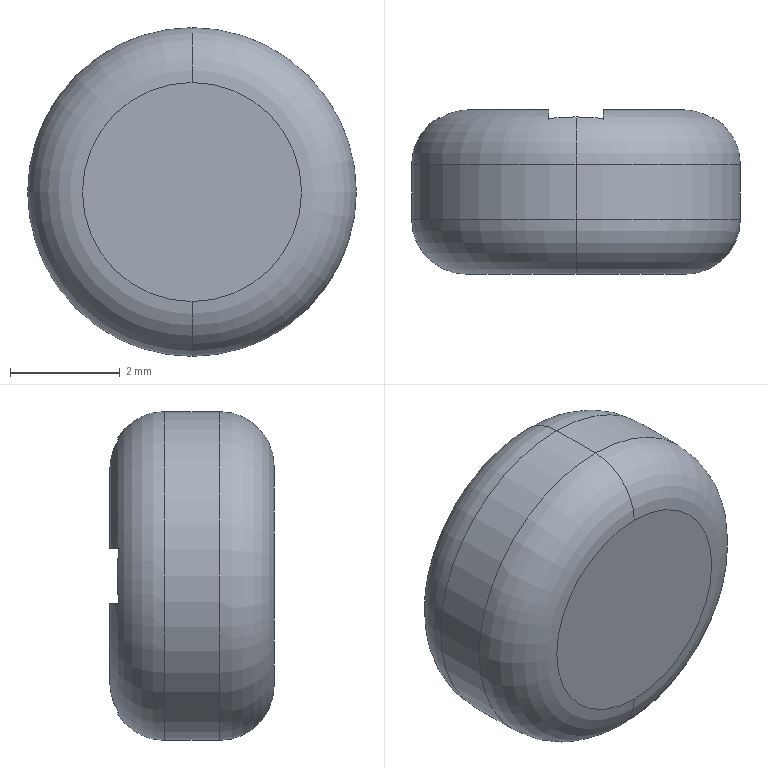Part | SolidWorks | features BaseBody 1 | 1 solid | 24 faces | box 6 x 3 x 6 mm | volume 63.932 mm3 | plane 18 | torus 4 | cylinder 2 | commonest cylinder face diameters 6 x2
STEP:
#1=CARTESIAN_POINT('',(0.,0.,-2.));
#2=VERTEX_POINT('',#1);
#3=CARTESIAN_POINT('',(0.,0.,2.));
#4=VERTEX_POINT('',#3);
#5=CARTESIAN_POINT('',(0.,0.,0.));
#6=DIRECTION('',(0.,-1.,0.));
#7=DIRECTION('',(0.,0.,1.));
#8=AXIS2_PLACEMENT_3D('',#5,#6,#7);
#9=CIRCLE('',#8,2.);
#10=EDGE_CURVE('',#2,#4,#9,.T.);
#11=ORIENTED_EDGE('',*,*,#10,.F.);
#12=CARTESIAN_POINT('',(0.,1.,-3.));
#13=VERTEX_POINT('',#12);
#14=CARTESIAN_POINT('',(0.,1.,-2.));
#15=DIRECTION('',(1.,0.,0.));
#16=DIRECTION('',(0.,0.,-1.));
#17=AXIS2_PLACEMENT_3D('',#14,#15,#16);
#18=CIRCLE('',#17,1.);
#19=EDGE_CURVE('',#2,#13,#18,.T.);
#20=ORIENTED_EDGE('',*,*,#19,.T.);
#21=CARTESIAN_POINT('',(0.,1.,3.));
#22=VERTEX_POINT('',#21);
#23=CARTESIAN_POINT('',(0.,1.,0.));
#24=DIRECTION('',(0.,1.,0.));
#25=DIRECTION('',(0.,0.,1.));
#26=AXIS2_PLACEMENT_3D('',#23,#24,#25);
#27=CIRCLE('',#26,3.);
#28=EDGE_CURVE('',#22,#13,#27,.T.);
#29=ORIENTED_EDGE('',*,*,#28,.F.);
#30=CARTESIAN_POINT('',(0.,1.,2.));
#31=DIRECTION('',(-1.,0.,0.));
#32=DIRECTION('',(0.,0.,1.));
#33=AXIS2_PLACEMENT_3D('',#30,#31,#32);
#34=CIRCLE('',#33,1.);
#35=EDGE_CURVE('',#4,#22,#34,.T.);
#36=ORIENTED_EDGE('',*,*,#35,.F.);
#37=EDGE_LOOP('',(#11,#20,#29,#36));
#38=FACE_OUTER_BOUND('',#37,.T.);
#39=CARTESIAN_POINT('',(0.,1.,0.));
#40=DIRECTION('',(0.,1.,0.));
#41=DIRECTION('',(0.,0.,1.));
#42=AXIS2_PLACEMENT_3D('',#39,#40,#41);
#43=TOROIDAL_SURFACE('',#42,2.,1.);
#44=ADVANCED_FACE('',(#38),#43,.T.);
#45=CARTESIAN_POINT('',(0.,2.,-3.));
#46=VERTEX_POINT('',#45);
#47=CARTESIAN_POINT('',(0.,2.,3.));
#48=VERTEX_POINT('',#47);
#49=CARTESIAN_POINT('',(0.,2.,0.));
#50=DIRECTION('',(0.,-1.,0.));
#51=DIRECTION('',(0.,0.,1.));
#52=AXIS2_PLACEMENT_3D('',#49,#50,#51);
#53=CIRCLE('',#52,3.);
#54=EDGE_CURVE('',#46,#48,#53,.T.);
#55=ORIENTED_EDGE('',*,*,#54,.T.);
#56=CARTESIAN_POINT('',(0.,3.,3.));
#57=DIRECTION('',(0.,-1.,0.));
#58=VECTOR('',#57,1000.);
#59=LINE('',#56,#58);
#60=EDGE_CURVE('',#48,#22,#59,.T.);
#61=ORIENTED_EDGE('',*,*,#60,.T.);
#62=ORIENTED_EDGE('',*,*,#28,.T.);
#63=CARTESIAN_POINT('',(0.,3.,-3.));
#64=DIRECTION('',(0.,-1.,0.));
#65=VECTOR('',#64,1000.);
#66=LINE('',#63,#65);
#67=EDGE_CURVE('',#46,#13,#66,.T.);
#68=ORIENTED_EDGE('',*,*,#67,.F.);
#69=EDGE_LOOP('',(#55,#61,#62,#68));
#70=FACE_OUTER_BOUND('',#69,.T.);
#71=CARTESIAN_POINT('',(0.,3.,0.));
#72=DIRECTION('',(0.,-1.,0.));
#73=DIRECTION('',(0.,0.,-1.));
#74=AXIS2_PLACEMENT_3D('',#71,#72,#73);
#75=CYLINDRICAL_SURFACE('',#74,3.);
#76=ADVANCED_FACE('',(#70),#75,.T.);
#77=ORIENTED_EDGE('',*,*,#54,.F.);
#78=CARTESIAN_POINT('',(0.,2.866,-2.5));
#79=VERTEX_POINT('',#78);
#80=CARTESIAN_POINT('',(0.,2.,-2.));
#81=DIRECTION('',(1.,0.,0.));
#82=DIRECTION('',(0.,0.,-1.));
#83=AXIS2_PLACEMENT_3D('',#80,#81,#82);
#84=CIRCLE('',#83,1.);
#85=EDGE_CURVE('',#46,#79,#84,.T.);
#86=ORIENTED_EDGE('',*,*,#85,.T.);
#87=CARTESIAN_POINT('',(0.5,2.835,-2.5));
#88=VERTEX_POINT('',#87);
#89=CARTESIAN_POINT('',(0.5,2.835,-2.5));
#90=CARTESIAN_POINT('',(0.4174,2.846,-2.5));
#91=CARTESIAN_POINT('',(0.3344,2.854,-2.5));
#92=CARTESIAN_POINT('',(0.1677,2.864,-2.5));
#93=CARTESIAN_POINT('',(0.08401,2.866,-2.5));
#94=CARTESIAN_POINT('',(0.,2.866,-2.5));
#95=B_SPLINE_CURVE_WITH_KNOTS('',3,(#89,#90,#91,#92,#93,#94),.UNSPECIFIED.,.F.,.F.,(4,2,4),(0.007633,0.007882,0.008131),.UNSPECIFIED.);
#96=EDGE_CURVE('',#88,#79,#95,.T.);
#97=ORIENTED_EDGE('',*,*,#96,.F.);
#98=CARTESIAN_POINT('',(0.5,3.,-1.936));
#99=VERTEX_POINT('',#98);
#100=CARTESIAN_POINT('',(0.5,3.,-1.936));
#101=CARTESIAN_POINT('',(0.5,3.,-2.136));
#102=CARTESIAN_POINT('',(0.5,2.944,-2.332));
#103=CARTESIAN_POINT('',(0.5,2.835,-2.5));
#104=B_SPLINE_CURVE_WITH_KNOTS('',3,(#100,#101,#102,#103),.UNSPECIFIED.,.F.,.F.,(4,4),(0.,1.),.UNSPECIFIED.);
#105=EDGE_CURVE('',#99,#88,#104,.T.);
#106=ORIENTED_EDGE('',*,*,#105,.F.);
#107=CARTESIAN_POINT('',(1.936,3.,-0.5));
#108=VERTEX_POINT('',#107);
#109=CARTESIAN_POINT('',(0.,3.,0.));
#110=DIRECTION('',(0.,1.,0.));
#111=DIRECTION('',(0.,0.,1.));
#112=AXIS2_PLACEMENT_3D('',#109,#110,#111);
#113=CIRCLE('',#112,2.);
#114=EDGE_CURVE('',#108,#99,#113,.T.);
#115=ORIENTED_EDGE('',*,*,#114,.F.);
#116=CARTESIAN_POINT('',(2.5,2.835,-0.5));
#117=VERTEX_POINT('',#116);
#118=CARTESIAN_POINT('',(2.5,2.835,-0.5));
#119=CARTESIAN_POINT('',(2.459,2.862,-0.5));
#120=CARTESIAN_POINT('',(2.416,2.886,-0.5));
#121=CARTESIAN_POINT('',(2.326,2.927,-0.5));
#122=CARTESIAN_POINT('',(2.277,2.944,-0.5));
#123=CARTESIAN_POINT('',(2.136,2.986,-0.5));
#124=CARTESIAN_POINT('',(2.038,3.,-0.5));
#125=CARTESIAN_POINT('',(1.936,3.,-0.5));
#126=B_SPLINE_CURVE_WITH_KNOTS('',3,(#118,#119,#120,#121,#122,#123,#124,#125),.UNSPECIFIED.,.F.,.F.,(4,2,2,4),(0.,0.25,0.5,1.),.UNSPECIFIED.);
#127=EDGE_CURVE('',#117,#108,#126,.T.);
#128=ORIENTED_EDGE('',*,*,#127,.F.);
#129=CARTESIAN_POINT('',(2.5,2.835,0.5));
#130=VERTEX_POINT('',#129);
#131=CARTESIAN_POINT('',(2.5,2.835,-0.5));
#132=CARTESIAN_POINT('',(2.5,2.857,-0.3347));
#133=CARTESIAN_POINT('',(2.5,2.866,-0.1698));
#134=CARTESIAN_POINT('',(2.5,2.866,0.1702));
#135=CARTESIAN_POINT('',(2.5,2.857,0.3348));
#136=CARTESIAN_POINT('',(2.5,2.835,0.5));
#137=B_SPLINE_CURVE_WITH_KNOTS('',3,(#131,#132,#133,#134,#135,#136),.UNSPECIFIED.,.F.,.F.,(4,2,4),(0.,0.5,1.),.UNSPECIFIED.);
#138=EDGE_CURVE('',#117,#130,#137,.T.);
#139=ORIENTED_EDGE('',*,*,#138,.T.);
#140=CARTESIAN_POINT('',(1.936,3.,0.5));
#141=VERTEX_POINT('',#140);
#142=CARTESIAN_POINT('',(2.5,2.835,0.5));
#143=CARTESIAN_POINT('',(2.323,2.95,0.5));
#144=CARTESIAN_POINT('',(2.122,3.,0.5));
#145=CARTESIAN_POINT('',(1.936,3.,0.5));
#146=B_SPLINE_CURVE_WITH_KNOTS('',3,(#142,#143,#144,#145),.UNSPECIFIED.,.F.,.F.,(4,4),(0.,1.),.UNSPECIFIED.);
#147=EDGE_CURVE('',#130,#141,#146,.T.);
#148=ORIENTED_EDGE('',*,*,#147,.T.);
#149=CARTESIAN_POINT('',(0.5,3.,1.936));
#150=VERTEX_POINT('',#149);
#151=CARTESIAN_POINT('',(0.,3.,0.));
#152=DIRECTION('',(0.,1.,0.));
#153=DIRECTION('',(0.,0.,1.));
#154=AXIS2_PLACEMENT_3D('',#151,#152,#153);
#155=CIRCLE('',#154,2.);
#156=EDGE_CURVE('',#150,#141,#155,.T.);
#157=ORIENTED_EDGE('',*,*,#156,.F.);
#158=CARTESIAN_POINT('',(0.5,2.835,2.5));
#159=VERTEX_POINT('',#158);
#160=CARTESIAN_POINT('',(0.5,2.835,2.5));
#161=CARTESIAN_POINT('',(0.5,2.862,2.459));
#162=CARTESIAN_POINT('',(0.5,2.886,2.416));
#163=CARTESIAN_POINT('',(0.5,2.927,2.326));
#164=CARTESIAN_POINT('',(0.5,2.944,2.277));
#165=CARTESIAN_POINT('',(0.5,2.986,2.136));
#166=CARTESIAN_POINT('',(0.5,3.,2.038));
#167=CARTESIAN_POINT('',(0.5,3.,1.936));
#168=B_SPLINE_CURVE_WITH_KNOTS('',3,(#160,#161,#162,#163,#164,#165,#166,#167),.UNSPECIFIED.,.F.,.F.,(4,2,2,4),(0.,0.25,0.5,1.),.UNSPECIFIED.);
#169=EDGE_CURVE('',#159,#150,#168,.T.);
#170=ORIENTED_EDGE('',*,*,#169,.F.);
#171=CARTESIAN_POINT('',(0.,2.866,2.5));
#172=VERTEX_POINT('',#171);
#173=CARTESIAN_POINT('',(0.5,2.835,2.5));
#174=CARTESIAN_POINT('',(0.4174,2.846,2.5));
#175=CARTESIAN_POINT('',(0.3344,2.854,2.5));
#176=CARTESIAN_POINT('',(0.1677,2.864,2.5));
#177=CARTESIAN_POINT('',(0.08401,2.866,2.5));
#178=CARTESIAN_POINT('',(0.,2.866,2.5));
#179=B_SPLINE_CURVE_WITH_KNOTS('',3,(#173,#174,#175,#176,#177,#178),.UNSPECIFIED.,.F.,.F.,(4,2,4),(0.007633,0.007882,0.008131),.UNSPECIFIED.);
#180=EDGE_CURVE('',#159,#172,#179,.T.);
#181=ORIENTED_EDGE('',*,*,#180,.T.);
#182=CARTESIAN_POINT('',(0.,2.,2.));
#183=DIRECTION('',(-1.,0.,0.));
#184=DIRECTION('',(0.,0.,1.));
#185=AXIS2_PLACEMENT_3D('',#182,#183,#184);
#186=CIRCLE('',#185,1.);
#187=EDGE_CURVE('',#48,#172,#186,.T.);
#188=ORIENTED_EDGE('',*,*,#187,.F.);
#189=EDGE_LOOP('',(#77,#86,#97,#106,#115,#128,#139,#148,#157,#170,#181,#188));
#190=FACE_OUTER_BOUND('',#189,.T.);
#191=CARTESIAN_POINT('',(0.,2.,0.));
#192=DIRECTION('',(0.,1.,0.));
#193=DIRECTION('',(0.,0.,1.));
#194=AXIS2_PLACEMENT_3D('',#191,#192,#193);
#195=TOROIDAL_SURFACE('',#194,2.,1.);
#196=ADVANCED_FACE('',(#190),#195,.T.);
#197=CARTESIAN_POINT('',(-1.936,3.,0.5));
#198=VERTEX_POINT('',#197);
#199=CARTESIAN_POINT('',(-0.5,3.,1.936));
#200=VERTEX_POINT('',#199);
#201=CARTESIAN_POINT('',(0.,3.,0.));
#202=DIRECTION('',(0.,1.,0.));
#203=DIRECTION('',(0.,0.,1.));
#204=AXIS2_PLACEMENT_3D('',#201,#202,#203);
#205=CIRCLE('',#204,2.);
#206=EDGE_CURVE('',#198,#200,#205,.T.);
#207=ORIENTED_EDGE('',*,*,#206,.T.);
#208=CARTESIAN_POINT('',(-0.5,3.,0.5));
#209=VERTEX_POINT('',#208);
#210=CARTESIAN_POINT('',(-0.5,3.,-0.02036));
#211=DIRECTION('',(0.,0.,-1.));
#212=VECTOR('',#211,1000.);
#213=LINE('',#210,#212);
#214=EDGE_CURVE('',#200,#209,#213,.T.);
#215=ORIENTED_EDGE('',*,*,#214,.T.);
#216=CARTESIAN_POINT('',(-4.826,3.,0.5));
#217=DIRECTION('',(-1.,0.,0.));
#218=VECTOR('',#217,1000.);
#219=LINE('',#216,#218);
#220=EDGE_CURVE('',#209,#198,#219,.T.);
#221=ORIENTED_EDGE('',*,*,#220,.T.);
#222=EDGE_LOOP('',(#207,#215,#221));
#223=FACE_OUTER_BOUND('',#222,.T.);
#224=CARTESIAN_POINT('',(0.,3.,0.));
#225=DIRECTION('',(0.,1.,0.));
#226=DIRECTION('',(1.,0.,0.));
#227=AXIS2_PLACEMENT_3D('',#224,#225,#226);
#228=PLANE('',#227);
#229=ADVANCED_FACE('',(#223),#228,.T.);
#230=CARTESIAN_POINT('',(-0.5,3.,-0.5));
#231=VERTEX_POINT('',#230);
#232=CARTESIAN_POINT('',(-1.936,3.,-0.5));
#233=VERTEX_POINT('',#232);
#234=CARTESIAN_POINT('',(-4.826,3.,-0.5));
#235=DIRECTION('',(-1.,0.,0.));
#236=VECTOR('',#235,1000.);
#237=LINE('',#234,#236);
#238=EDGE_CURVE('',#231,#233,#237,.T.);
#239=ORIENTED_EDGE('',*,*,#238,.F.);
#240=CARTESIAN_POINT('',(-0.5,3.,-1.936));
#241=VERTEX_POINT('',#240);
#242=CARTESIAN_POINT('',(-0.5,3.,-0.02036));
#243=DIRECTION('',(0.,0.,-1.));
#244=VECTOR('',#243,1000.);
#245=LINE('',#242,#244);
#246=EDGE_CURVE('',#231,#241,#245,.T.);
#247=ORIENTED_EDGE('',*,*,#246,.T.);
#248=CARTESIAN_POINT('',(0.,3.,0.));
#249=DIRECTION('',(0.,1.,0.));
#250=DIRECTION('',(0.,0.,1.));
#251=AXIS2_PLACEMENT_3D('',#248,#249,#250);
#252=CIRCLE('',#251,2.);
#253=EDGE_CURVE('',#241,#233,#252,.T.);
#254=ORIENTED_EDGE('',*,*,#253,.T.);
#255=EDGE_LOOP('',(#239,#247,#254));
#256=FACE_OUTER_BOUND('',#255,.T.);
#257=CARTESIAN_POINT('',(0.,3.,0.));
#258=DIRECTION('',(0.,1.,0.));
#259=DIRECTION('',(1.,0.,0.));
#260=AXIS2_PLACEMENT_3D('',#257,#258,#259);
#261=PLANE('',#260);
#262=ADVANCED_FACE('',(#256),#261,.T.);
#263=ORIENTED_EDGE('',*,*,#156,.T.);
#264=CARTESIAN_POINT('',(0.5,3.,0.5));
#265=VERTEX_POINT('',#264);
#266=CARTESIAN_POINT('',(-4.826,3.,0.5));
#267=DIRECTION('',(-1.,0.,0.));
#268=VECTOR('',#267,1000.);
#269=LINE('',#266,#268);
#270=EDGE_CURVE('',#141,#265,#269,.T.);
#271=ORIENTED_EDGE('',*,*,#270,.T.);
#272=CARTESIAN_POINT('',(0.5,3.,-0.02036));
#273=DIRECTION('',(0.,0.,-1.));
#274=VECTOR('',#273,1000.);
#275=LINE('',#272,#274);
#276=EDGE_CURVE('',#150,#265,#275,.T.);
#277=ORIENTED_EDGE('',*,*,#276,.F.);
#278=EDGE_LOOP('',(#263,#271,#277));
#279=FACE_OUTER_BOUND('',#278,.T.);
#280=CARTESIAN_POINT('',(0.,3.,0.));
#281=DIRECTION('',(0.,1.,0.));
#282=DIRECTION('',(1.,0.,0.));
#283=AXIS2_PLACEMENT_3D('',#280,#281,#282);
#284=PLANE('',#283);
#285=ADVANCED_FACE('',(#279),#284,.T.);
#286=ORIENTED_EDGE('',*,*,#85,.F.);
#287=CARTESIAN_POINT('',(0.,2.,0.));
#288=DIRECTION('',(0.,-1.,0.));
#289=DIRECTION('',(0.,0.,1.));
#290=AXIS2_PLACEMENT_3D('',#287,#288,#289);
#291=CIRCLE('',#290,3.);
#292=EDGE_CURVE('',#48,#46,#291,.T.);
#293=ORIENTED_EDGE('',*,*,#292,.F.);
#294=ORIENTED_EDGE('',*,*,#187,.T.);
#295=CARTESIAN_POINT('',(-0.5,2.835,2.5));
#296=VERTEX_POINT('',#295);
#297=CARTESIAN_POINT('',(0.,2.866,2.5));
#298=CARTESIAN_POINT('',(-0.08407,2.866,2.5));
#299=CARTESIAN_POINT('',(-0.1678,2.864,2.5));
#300=CARTESIAN_POINT('',(-0.3345,2.854,2.5));
#301=CARTESIAN_POINT('',(-0.4175,2.846,2.5));
#302=CARTESIAN_POINT('',(-0.5,2.835,2.5));
#303=B_SPLINE_CURVE_WITH_KNOTS('',3,(#297,#298,#299,#300,#301,#302),.UNSPECIFIED.,.F.,.F.,(4,2,4),(0.,0.0002496,0.0004992),.UNSPECIFIED.);
#304=EDGE_CURVE('',#172,#296,#303,.T.);
#305=ORIENTED_EDGE('',*,*,#304,.T.);
#306=CARTESIAN_POINT('',(-0.5,2.835,2.5));
#307=CARTESIAN_POINT('',(-0.5,2.95,2.323));
#308=CARTESIAN_POINT('',(-0.5,3.,2.122));
#309=CARTESIAN_POINT('',(-0.5,3.,1.936));
#310=B_SPLINE_CURVE_WITH_KNOTS('',3,(#306,#307,#308,#309),.UNSPECIFIED.,.F.,.F.,(4,4),(0.,1.),.UNSPECIFIED.);
#311=EDGE_CURVE('',#296,#200,#310,.T.);
#312=ORIENTED_EDGE('',*,*,#311,.T.);
#313=ORIENTED_EDGE('',*,*,#206,.F.);
#314=CARTESIAN_POINT('',(-2.5,2.835,0.5));
#315=VERTEX_POINT('',#314);
#316=CARTESIAN_POINT('',(-1.936,3.,0.5));
#317=CARTESIAN_POINT('',(-2.122,3.,0.5));
#318=CARTESIAN_POINT('',(-2.323,2.95,0.5));
#319=CARTESIAN_POINT('',(-2.5,2.835,0.5));
#320=B_SPLINE_CURVE_WITH_KNOTS('',3,(#316,#317,#318,#319),.UNSPECIFIED.,.F.,.F.,(4,4),(0.,1.),.UNSPECIFIED.);
#321=EDGE_CURVE('',#198,#315,#320,.T.);
#322=ORIENTED_EDGE('',*,*,#321,.T.);
#323=CARTESIAN_POINT('',(-2.5,2.835,-0.5));
#324=VERTEX_POINT('',#323);
#325=CARTESIAN_POINT('',(-2.5,2.835,-0.5));
#326=CARTESIAN_POINT('',(-2.5,2.856,-0.3424));
#327=CARTESIAN_POINT('',(-2.5,2.866,-0.1749));
#328=CARTESIAN_POINT('',(-2.5,2.866,0.1753));
#329=CARTESIAN_POINT('',(-2.5,2.856,0.3419));
#330=CARTESIAN_POINT('',(-2.5,2.835,0.5));
#331=B_SPLINE_CURVE_WITH_KNOTS('',3,(#325,#326,#327,#328,#329,#330),.UNSPECIFIED.,.F.,.F.,(4,2,4),(0.,0.5,1.),.UNSPECIFIED.);
#332=EDGE_CURVE('',#324,#315,#331,.T.);
#333=ORIENTED_EDGE('',*,*,#332,.F.);
#334=CARTESIAN_POINT('',(-1.936,3.,-0.5));
#335=CARTESIAN_POINT('',(-2.136,3.,-0.5));
#336=CARTESIAN_POINT('',(-2.332,2.944,-0.5));
#337=CARTESIAN_POINT('',(-2.5,2.835,-0.5));
#338=B_SPLINE_CURVE_WITH_KNOTS('',3,(#334,#335,#336,#337),.UNSPECIFIED.,.F.,.F.,(4,4),(0.,1.),.UNSPECIFIED.);
#339=EDGE_CURVE('',#233,#324,#338,.T.);
#340=ORIENTED_EDGE('',*,*,#339,.F.);
#341=ORIENTED_EDGE('',*,*,#253,.F.);
#342=CARTESIAN_POINT('',(-0.5,2.835,-2.5));
#343=VERTEX_POINT('',#342);
#344=CARTESIAN_POINT('',(-0.5,3.,-1.936));
#345=CARTESIAN_POINT('',(-0.5,3.,-2.122));
#346=CARTESIAN_POINT('',(-0.5,2.95,-2.323));
#347=CARTESIAN_POINT('',(-0.5,2.835,-2.5));
#348=B_SPLINE_CURVE_WITH_KNOTS('',3,(#344,#345,#346,#347),.UNSPECIFIED.,.F.,.F.,(4,4),(0.,1.),.UNSPECIFIED.);
#349=EDGE_CURVE('',#241,#343,#348,.T.);
#350=ORIENTED_EDGE('',*,*,#349,.T.);
#351=CARTESIAN_POINT('',(0.,2.866,-2.5));
#352=CARTESIAN_POINT('',(-0.08407,2.866,-2.5));
#353=CARTESIAN_POINT('',(-0.1678,2.864,-2.5));
#354=CARTESIAN_POINT('',(-0.3345,2.854,-2.5));
#355=CARTESIAN_POINT('',(-0.4175,2.846,-2.5));
#356=CARTESIAN_POINT('',(-0.5,2.835,-2.5));
#357=B_SPLINE_CURVE_WITH_KNOTS('',3,(#351,#352,#353,#354,#355,#356),.UNSPECIFIED.,.F.,.F.,(4,2,4),(0.,0.0002496,0.0004992),.UNSPECIFIED.);
#358=EDGE_CURVE('',#79,#343,#357,.T.);
#359=ORIENTED_EDGE('',*,*,#358,.F.);
#360=EDGE_LOOP('',(#286,#293,#294,#305,#312,#313,#322,#333,#340,#341,#350,#359));
#361=FACE_OUTER_BOUND('',#360,.T.);
#362=CARTESIAN_POINT('',(0.,2.,0.));
#363=DIRECTION('',(0.,1.,0.));
#364=DIRECTION('',(0.,0.,1.));
#365=AXIS2_PLACEMENT_3D('',#362,#363,#364);
#366=TOROIDAL_SURFACE('',#365,2.,1.);
#367=ADVANCED_FACE('',(#361),#366,.T.);
#368=ORIENTED_EDGE('',*,*,#60,.F.);
#369=ORIENTED_EDGE('',*,*,#292,.T.);
#370=ORIENTED_EDGE('',*,*,#67,.T.);
#371=CARTESIAN_POINT('',(0.,1.,0.));
#372=DIRECTION('',(0.,1.,0.));
#373=DIRECTION('',(0.,0.,1.));
#374=AXIS2_PLACEMENT_3D('',#371,#372,#373);
#375=CIRCLE('',#374,3.);
#376=EDGE_CURVE('',#13,#22,#375,.T.);
#377=ORIENTED_EDGE('',*,*,#376,.T.);
#378=EDGE_LOOP('',(#368,#369,#370,#377));
#379=FACE_OUTER_BOUND('',#378,.T.);
#380=CARTESIAN_POINT('',(0.,3.,0.));
#381=DIRECTION('',(0.,-1.,0.));
#382=DIRECTION('',(0.,0.,-1.));
#383=AXIS2_PLACEMENT_3D('',#380,#381,#382);
#384=CYLINDRICAL_SURFACE('',#383,3.);
#385=ADVANCED_FACE('',(#379),#384,.T.);
#386=CARTESIAN_POINT('',(0.5,3.,-0.5));
#387=VERTEX_POINT('',#386);
#388=CARTESIAN_POINT('',(0.5,3.,-0.02036));
#389=DIRECTION('',(0.,0.,-1.));
#390=VECTOR('',#389,1000.);
#391=LINE('',#388,#390);
#392=EDGE_CURVE('',#387,#99,#391,.T.);
#393=ORIENTED_EDGE('',*,*,#392,.F.);
#394=CARTESIAN_POINT('',(-4.826,3.,-0.5));
#395=DIRECTION('',(-1.,0.,0.));
#396=VECTOR('',#395,1000.);
#397=LINE('',#394,#396);
#398=EDGE_CURVE('',#108,#387,#397,.T.);
#399=ORIENTED_EDGE('',*,*,#398,.F.);
#400=ORIENTED_EDGE('',*,*,#114,.T.);
#401=EDGE_LOOP('',(#393,#399,#400));
#402=FACE_OUTER_BOUND('',#401,.T.);
#403=CARTESIAN_POINT('',(0.,3.,0.));
#404=DIRECTION('',(0.,1.,0.));
#405=DIRECTION('',(1.,0.,0.));
#406=AXIS2_PLACEMENT_3D('',#403,#404,#405);
#407=PLANE('',#406);
#408=ADVANCED_FACE('',(#402),#407,.T.);
#409=CARTESIAN_POINT('',(0.,0.,0.));
#410=DIRECTION('',(0.,-1.,0.));
#411=DIRECTION('',(0.,0.,1.));
#412=AXIS2_PLACEMENT_3D('',#409,#410,#411);
#413=CIRCLE('',#412,2.);
#414=EDGE_CURVE('',#4,#2,#413,.T.);
#415=ORIENTED_EDGE('',*,*,#414,.T.);
#416=ORIENTED_EDGE('',*,*,#10,.T.);
#417=EDGE_LOOP('',(#415,#416));
#418=FACE_OUTER_BOUND('',#417,.T.);
#419=CARTESIAN_POINT('',(0.,0.,0.));
#420=DIRECTION('',(0.,1.,0.));
#421=DIRECTION('',(1.,0.,0.));
#422=AXIS2_PLACEMENT_3D('',#419,#420,#421);
#423=PLANE('',#422);
#424=ADVANCED_FACE('',(#418),#423,.F.);
#425=ORIENTED_EDGE('',*,*,#19,.F.);
#426=ORIENTED_EDGE('',*,*,#414,.F.);
#427=ORIENTED_EDGE('',*,*,#35,.T.);
#428=ORIENTED_EDGE('',*,*,#376,.F.);
#429=EDGE_LOOP('',(#425,#426,#427,#428));
#430=FACE_OUTER_BOUND('',#429,.T.);
#431=CARTESIAN_POINT('',(0.,1.,0.));
#432=DIRECTION('',(0.,1.,0.));
#433=DIRECTION('',(0.,0.,1.));
#434=AXIS2_PLACEMENT_3D('',#431,#432,#433);
#435=TOROIDAL_SURFACE('',#434,2.,1.);
#436=ADVANCED_FACE('',(#430),#435,.T.);
#437=CARTESIAN_POINT('',(-0.5,1.5,2.5));
#438=VERTEX_POINT('',#437);
#439=CARTESIAN_POINT('',(-0.5,1.5,2.5));
#440=DIRECTION('',(0.,1.,0.));
#441=VECTOR('',#440,1000.);
#442=LINE('',#439,#441);
#443=EDGE_CURVE('',#438,#296,#442,.T.);
#444=ORIENTED_EDGE('',*,*,#443,.F.);
#445=CARTESIAN_POINT('',(-0.5,1.5,0.5));
#446=VERTEX_POINT('',#445);
#447=CARTESIAN_POINT('',(-0.5,1.5,-0.02036));
#448=DIRECTION('',(0.,0.,-1.));
#449=VECTOR('',#448,1000.);
#450=LINE('',#447,#449);
#451=EDGE_CURVE('',#438,#446,#450,.T.);
#452=ORIENTED_EDGE('',*,*,#451,.T.);
#453=CARTESIAN_POINT('',(-0.5,1.5,0.5));
#454=DIRECTION('',(0.,1.,0.));
#455=VECTOR('',#454,1000.);
#456=LINE('',#453,#455);
#457=EDGE_CURVE('',#446,#209,#456,.T.);
#458=ORIENTED_EDGE('',*,*,#457,.T.);
#459=ORIENTED_EDGE('',*,*,#214,.F.);
#460=ORIENTED_EDGE('',*,*,#311,.F.);
#461=EDGE_LOOP('',(#444,#452,#458,#459,#460));
#462=FACE_OUTER_BOUND('',#461,.T.);
#463=CARTESIAN_POINT('',(-0.5,1.5,-0.02036));
#464=DIRECTION('',(1.,0.,0.));
#465=DIRECTION('',(0.,0.,-1.));
#466=AXIS2_PLACEMENT_3D('',#463,#464,#465);
#467=PLANE('',#466);
#468=ADVANCED_FACE('',(#462),#467,.T.);
#469=ORIENTED_EDGE('',*,*,#220,.F.);
#470=ORIENTED_EDGE('',*,*,#457,.F.);
#471=CARTESIAN_POINT('',(-2.5,1.5,0.5));
#472=VERTEX_POINT('',#471);
#473=CARTESIAN_POINT('',(-4.826,1.5,0.5));
#474=DIRECTION('',(-1.,0.,0.));
#475=VECTOR('',#474,1000.);
#476=LINE('',#473,#475);
#477=EDGE_CURVE('',#446,#472,#476,.T.);
#478=ORIENTED_EDGE('',*,*,#477,.T.);
#479=CARTESIAN_POINT('',(-2.5,1.5,0.5));
#480=DIRECTION('',(0.,1.,0.));
#481=VECTOR('',#480,1000.);
#482=LINE('',#479,#481);
#483=EDGE_CURVE('',#472,#315,#482,.T.);
#484=ORIENTED_EDGE('',*,*,#483,.T.);
#485=ORIENTED_EDGE('',*,*,#321,.F.);
#486=EDGE_LOOP('',(#469,#470,#478,#484,#485));
#487=FACE_OUTER_BOUND('',#486,.T.);
#488=CARTESIAN_POINT('',(-4.826,1.5,0.5));
#489=DIRECTION('',(0.,0.,-1.));
#490=DIRECTION('',(-1.,0.,0.));
#491=AXIS2_PLACEMENT_3D('',#488,#489,#490);
#492=PLANE('',#491);
#493=ADVANCED_FACE('',(#487),#492,.T.);
#494=ORIENTED_EDGE('',*,*,#332,.T.);
#495=ORIENTED_EDGE('',*,*,#483,.F.);
#496=CARTESIAN_POINT('',(-2.5,1.5,-0.5));
#497=VERTEX_POINT('',#496);
#498=CARTESIAN_POINT('',(-2.5,1.5,-0.02036));
#499=DIRECTION('',(0.,0.,1.));
#500=VECTOR('',#499,1000.);
#501=LINE('',#498,#500);
#502=EDGE_CURVE('',#497,#472,#501,.T.);
#503=ORIENTED_EDGE('',*,*,#502,.F.);
#504=CARTESIAN_POINT('',(-2.5,1.5,-0.5));
#505=DIRECTION('',(0.,1.,0.));
#506=VECTOR('',#505,1000.);
#507=LINE('',#504,#506);
#508=EDGE_CURVE('',#497,#324,#507,.T.);
#509=ORIENTED_EDGE('',*,*,#508,.T.);
#510=EDGE_LOOP('',(#494,#495,#503,#509));
#511=FACE_OUTER_BOUND('',#510,.T.);
#512=CARTESIAN_POINT('',(-2.5,1.5,-0.02036));
#513=DIRECTION('',(-1.,0.,0.));
#514=DIRECTION('',(0.,0.,1.));
#515=AXIS2_PLACEMENT_3D('',#512,#513,#514);
#516=PLANE('',#515);
#517=ADVANCED_FACE('',(#511),#516,.F.);
#518=ORIENTED_EDGE('',*,*,#339,.T.);
#519=ORIENTED_EDGE('',*,*,#508,.F.);
#520=CARTESIAN_POINT('',(-0.5,1.5,-0.5));
#521=VERTEX_POINT('',#520);
#522=CARTESIAN_POINT('',(-4.826,1.5,-0.5));
#523=DIRECTION('',(-1.,0.,0.));
#524=VECTOR('',#523,1000.);
#525=LINE('',#522,#524);
#526=EDGE_CURVE('',#521,#497,#525,.T.);
#527=ORIENTED_EDGE('',*,*,#526,.F.);
#528=CARTESIAN_POINT('',(-0.5,1.5,-0.5));
#529=DIRECTION('',(0.,1.,0.));
#530=VECTOR('',#529,1000.);
#531=LINE('',#528,#530);
#532=EDGE_CURVE('',#521,#231,#531,.T.);
#533=ORIENTED_EDGE('',*,*,#532,.T.);
#534=ORIENTED_EDGE('',*,*,#238,.T.);
#535=EDGE_LOOP('',(#518,#519,#527,#533,#534));
#536=FACE_OUTER_BOUND('',#535,.T.);
#537=CARTESIAN_POINT('',(-4.826,1.5,-0.5));
#538=DIRECTION('',(0.,0.,-1.));
#539=DIRECTION('',(-1.,0.,0.));
#540=AXIS2_PLACEMENT_3D('',#537,#538,#539);
#541=PLANE('',#540);
#542=ADVANCED_FACE('',(#536),#541,.F.);
#543=ORIENTED_EDGE('',*,*,#246,.F.);
#544=ORIENTED_EDGE('',*,*,#532,.F.);
#545=CARTESIAN_POINT('',(-0.5,1.5,-2.5));
#546=VERTEX_POINT('',#545);
#547=CARTESIAN_POINT('',(-0.5,1.5,-0.02036));
#548=DIRECTION('',(0.,0.,-1.));
#549=VECTOR('',#548,1000.);
#550=LINE('',#547,#549);
#551=EDGE_CURVE('',#521,#546,#550,.T.);
#552=ORIENTED_EDGE('',*,*,#551,.T.);
#553=CARTESIAN_POINT('',(-0.5,1.5,-2.5));
#554=DIRECTION('',(0.,1.,0.));
#555=VECTOR('',#554,1000.);
#556=LINE('',#553,#555);
#557=EDGE_CURVE('',#546,#343,#556,.T.);
#558=ORIENTED_EDGE('',*,*,#557,.T.);
#559=ORIENTED_EDGE('',*,*,#349,.F.);
#560=EDGE_LOOP('',(#543,#544,#552,#558,#559));
#561=FACE_OUTER_BOUND('',#560,.T.);
#562=CARTESIAN_POINT('',(-0.5,1.5,-0.02036));
#563=DIRECTION('',(1.,0.,0.));
#564=DIRECTION('',(0.,0.,-1.));
#565=AXIS2_PLACEMENT_3D('',#562,#563,#564);
#566=PLANE('',#565);
#567=ADVANCED_FACE('',(#561),#566,.T.);
#568=ORIENTED_EDGE('',*,*,#96,.T.);
#569=ORIENTED_EDGE('',*,*,#358,.T.);
#570=ORIENTED_EDGE('',*,*,#557,.F.);
#571=CARTESIAN_POINT('',(0.5,1.5,-2.5));
#572=VERTEX_POINT('',#571);
#573=CARTESIAN_POINT('',(-4.826,1.5,-2.5));
#574=DIRECTION('',(-1.,0.,0.));
#575=VECTOR('',#574,1000.);
#576=LINE('',#573,#575);
#577=EDGE_CURVE('',#572,#546,#576,.T.);
#578=ORIENTED_EDGE('',*,*,#577,.F.);
#579=CARTESIAN_POINT('',(0.5,1.5,-2.5));
#580=DIRECTION('',(0.,1.,0.));
#581=VECTOR('',#580,1000.);
#582=LINE('',#579,#581);
#583=EDGE_CURVE('',#572,#88,#582,.T.);
#584=ORIENTED_EDGE('',*,*,#583,.T.);
#585=EDGE_LOOP('',(#568,#569,#570,#578,#584));
#586=FACE_OUTER_BOUND('',#585,.T.);
#587=CARTESIAN_POINT('',(-4.826,1.5,-2.5));
#588=DIRECTION('',(0.,0.,-1.));
#589=DIRECTION('',(0.,-1.,0.));
#590=AXIS2_PLACEMENT_3D('',#587,#588,#589);
#591=PLANE('',#590);
#592=ADVANCED_FACE('',(#586),#591,.F.);
#593=ORIENTED_EDGE('',*,*,#105,.T.);
#594=ORIENTED_EDGE('',*,*,#583,.F.);
#595=CARTESIAN_POINT('',(0.5,1.5,-0.5));
#596=VERTEX_POINT('',#595);
#597=CARTESIAN_POINT('',(0.5,1.5,-0.02036));
#598=DIRECTION('',(0.,0.,-1.));
#599=VECTOR('',#598,1000.);
#600=LINE('',#597,#599);
#601=EDGE_CURVE('',#596,#572,#600,.T.);
#602=ORIENTED_EDGE('',*,*,#601,.F.);
#603=CARTESIAN_POINT('',(0.5,1.5,-0.5));
#604=DIRECTION('',(0.,1.,0.));
#605=VECTOR('',#604,1000.);
#606=LINE('',#603,#605);
#607=EDGE_CURVE('',#596,#387,#606,.T.);
#608=ORIENTED_EDGE('',*,*,#607,.T.);
#609=ORIENTED_EDGE('',*,*,#392,.T.);
#610=EDGE_LOOP('',(#593,#594,#602,#608,#609));
#611=FACE_OUTER_BOUND('',#610,.T.);
#612=CARTESIAN_POINT('',(0.5,1.5,-0.02036));
#613=DIRECTION('',(1.,0.,0.));
#614=DIRECTION('',(0.,1.,0.));
#615=AXIS2_PLACEMENT_3D('',#612,#613,#614);
#616=PLANE('',#615);
#617=ADVANCED_FACE('',(#611),#616,.F.);
#618=ORIENTED_EDGE('',*,*,#127,.T.);
#619=ORIENTED_EDGE('',*,*,#398,.T.);
#620=ORIENTED_EDGE('',*,*,#607,.F.);
#621=CARTESIAN_POINT('',(2.5,1.5,-0.5));
#622=VERTEX_POINT('',#621);
#623=CARTESIAN_POINT('',(-4.826,1.5,-0.5));
#624=DIRECTION('',(-1.,0.,0.));
#625=VECTOR('',#624,1000.);
#626=LINE('',#623,#625);
#627=EDGE_CURVE('',#622,#596,#626,.T.);
#628=ORIENTED_EDGE('',*,*,#627,.F.);
#629=CARTESIAN_POINT('',(2.5,1.5,-0.5));
#630=DIRECTION('',(0.,1.,0.));
#631=VECTOR('',#630,1000.);
#632=LINE('',#629,#631);
#633=EDGE_CURVE('',#622,#117,#632,.T.);
#634=ORIENTED_EDGE('',*,*,#633,.T.);
#635=EDGE_LOOP('',(#618,#619,#620,#628,#634));
#636=FACE_OUTER_BOUND('',#635,.T.);
#637=CARTESIAN_POINT('',(-4.826,1.5,-0.5));
#638=DIRECTION('',(0.,0.,-1.));
#639=DIRECTION('',(-1.,0.,0.));
#640=AXIS2_PLACEMENT_3D('',#637,#638,#639);
#641=PLANE('',#640);
#642=ADVANCED_FACE('',(#636),#641,.F.);
#643=ORIENTED_EDGE('',*,*,#633,.F.);
#644=CARTESIAN_POINT('',(2.5,1.5,0.5));
#645=VERTEX_POINT('',#644);
#646=CARTESIAN_POINT('',(2.5,1.5,-0.02036));
#647=DIRECTION('',(0.,0.,1.));
#648=VECTOR('',#647,1000.);
#649=LINE('',#646,#648);
#650=EDGE_CURVE('',#622,#645,#649,.T.);
#651=ORIENTED_EDGE('',*,*,#650,.T.);
#652=CARTESIAN_POINT('',(2.5,1.5,0.5));
#653=DIRECTION('',(0.,1.,0.));
#654=VECTOR('',#653,1000.);
#655=LINE('',#652,#654);
#656=EDGE_CURVE('',#645,#130,#655,.T.);
#657=ORIENTED_EDGE('',*,*,#656,.T.);
#658=ORIENTED_EDGE('',*,*,#138,.F.);
#659=EDGE_LOOP('',(#643,#651,#657,#658));
#660=FACE_OUTER_BOUND('',#659,.T.);
#661=CARTESIAN_POINT('',(2.5,1.5,-0.02036));
#662=DIRECTION('',(-1.,0.,0.));
#663=DIRECTION('',(0.,0.,1.));
#664=AXIS2_PLACEMENT_3D('',#661,#662,#663);
#665=PLANE('',#664);
#666=ADVANCED_FACE('',(#660),#665,.T.);
#667=ORIENTED_EDGE('',*,*,#656,.F.);
#668=CARTESIAN_POINT('',(0.5,1.5,0.5));
#669=VERTEX_POINT('',#668);
#670=CARTESIAN_POINT('',(-4.826,1.5,0.5));
#671=DIRECTION('',(-1.,0.,0.));
#672=VECTOR('',#671,1000.);
#673=LINE('',#670,#672);
#674=EDGE_CURVE('',#645,#669,#673,.T.);
#675=ORIENTED_EDGE('',*,*,#674,.T.);
#676=CARTESIAN_POINT('',(0.5,1.5,0.5));
#677=DIRECTION('',(0.,1.,0.));
#678=VECTOR('',#677,1000.);
#679=LINE('',#676,#678);
#680=EDGE_CURVE('',#669,#265,#679,.T.);
#681=ORIENTED_EDGE('',*,*,#680,.T.);
#682=ORIENTED_EDGE('',*,*,#270,.F.);
#683=ORIENTED_EDGE('',*,*,#147,.F.);
#684=EDGE_LOOP('',(#667,#675,#681,#682,#683));
#685=FACE_OUTER_BOUND('',#684,.T.);
#686=CARTESIAN_POINT('',(-4.826,1.5,0.5));
#687=DIRECTION('',(0.,0.,-1.));
#688=DIRECTION('',(-1.,0.,0.));
#689=AXIS2_PLACEMENT_3D('',#686,#687,#688);
#690=PLANE('',#689);
#691=ADVANCED_FACE('',(#685),#690,.T.);
#692=ORIENTED_EDGE('',*,*,#169,.T.);
#693=ORIENTED_EDGE('',*,*,#276,.T.);
#694=ORIENTED_EDGE('',*,*,#680,.F.);
#695=CARTESIAN_POINT('',(0.5,1.5,2.5));
#696=VERTEX_POINT('',#695);
#697=CARTESIAN_POINT('',(0.5,1.5,-0.02036));
#698=DIRECTION('',(0.,0.,-1.));
#699=VECTOR('',#698,1000.);
#700=LINE('',#697,#699);
#701=EDGE_CURVE('',#696,#669,#700,.T.);
#702=ORIENTED_EDGE('',*,*,#701,.F.);
#703=CARTESIAN_POINT('',(0.5,1.5,2.5));
#704=DIRECTION('',(0.,1.,0.));
#705=VECTOR('',#704,1000.);
#706=LINE('',#703,#705);
#707=EDGE_CURVE('',#696,#159,#706,.T.);
#708=ORIENTED_EDGE('',*,*,#707,.T.);
#709=EDGE_LOOP('',(#692,#693,#694,#702,#708));
#710=FACE_OUTER_BOUND('',#709,.T.);
#711=CARTESIAN_POINT('',(0.5,1.5,-0.02036));
#712=DIRECTION('',(1.,0.,0.));
#713=DIRECTION('',(0.,1.,0.));
#714=AXIS2_PLACEMENT_3D('',#711,#712,#713);
#715=PLANE('',#714);
#716=ADVANCED_FACE('',(#710),#715,.F.);
#717=ORIENTED_EDGE('',*,*,#707,.F.);
#718=CARTESIAN_POINT('',(-4.826,1.5,2.5));
#719=DIRECTION('',(-1.,0.,0.));
#720=VECTOR('',#719,1000.);
#721=LINE('',#718,#720);
#722=EDGE_CURVE('',#696,#438,#721,.T.);
#723=ORIENTED_EDGE('',*,*,#722,.T.);
#724=ORIENTED_EDGE('',*,*,#443,.T.);
#725=ORIENTED_EDGE('',*,*,#304,.F.);
#726=ORIENTED_EDGE('',*,*,#180,.F.);
#727=EDGE_LOOP('',(#717,#723,#724,#725,#726));
#728=FACE_OUTER_BOUND('',#727,.T.);
#729=CARTESIAN_POINT('',(-4.826,1.5,2.5));
#730=DIRECTION('',(0.,0.,-1.));
#731=DIRECTION('',(0.,-1.,0.));
#732=AXIS2_PLACEMENT_3D('',#729,#730,#731);
#733=PLANE('',#732);
#734=ADVANCED_FACE('',(#728),#733,.T.);
#735=ORIENTED_EDGE('',*,*,#451,.F.);
#736=ORIENTED_EDGE('',*,*,#722,.F.);
#737=ORIENTED_EDGE('',*,*,#701,.T.);
#738=ORIENTED_EDGE('',*,*,#674,.F.);
#739=ORIENTED_EDGE('',*,*,#650,.F.);
#740=ORIENTED_EDGE('',*,*,#627,.T.);
#741=ORIENTED_EDGE('',*,*,#601,.T.);
#742=ORIENTED_EDGE('',*,*,#577,.T.);
#743=ORIENTED_EDGE('',*,*,#551,.F.);
#744=ORIENTED_EDGE('',*,*,#526,.T.);
#745=ORIENTED_EDGE('',*,*,#502,.T.);
#746=ORIENTED_EDGE('',*,*,#477,.F.);
#747=EDGE_LOOP('',(#735,#736,#737,#738,#739,#740,#741,#742,#743,#744,#745,#746));
#748=FACE_OUTER_BOUND('',#747,.T.);
#749=CARTESIAN_POINT('',(-4.826,1.5,-0.02036));
#750=DIRECTION('',(0.,1.,0.));
#751=DIRECTION('',(1.,0.,0.));
#752=AXIS2_PLACEMENT_3D('',#749,#750,#751);
#753=PLANE('',#752);
#754=ADVANCED_FACE('',(#748),#753,.T.);
#755=CLOSED_SHELL('',(#44,#76,#196,#229,#262,#285,#367,#385,#408,#424,#436,#468,#493,#517,#542,#567,#592,#617,#642,#666,#691,#716,#734,#754));
#756=MANIFOLD_SOLID_BREP('',#755);
#757=CARTESIAN_POINT('',(0.,0.,0.));
#758=DIRECTION('',(0.,0.,1.));
#759=DIRECTION('',(1.,0.,0.));
#760=AXIS2_PLACEMENT_3D('',#757,#758,#759);
#761=(LENGTH_UNIT()NAMED_UNIT(*)SI_UNIT(.MILLI.,.METRE.));
#762=UNCERTAINTY_MEASURE_WITH_UNIT(LENGTH_MEASURE(0.00001),#761,'','');
#763=(NAMED_UNIT(*)PLANE_ANGLE_UNIT()SI_UNIT($,.RADIAN.));
#764=(NAMED_UNIT(*)SI_UNIT($,.STERADIAN.)SOLID_ANGLE_UNIT());
#765=(GEOMETRIC_REPRESENTATION_CONTEXT(3)GLOBAL_UNCERTAINTY_ASSIGNED_CONTEXT((#762))GLOBAL_UNIT_ASSIGNED_CONTEXT((#761,#763,#764))REPRESENTATION_CONTEXT('',''));
#766=ADVANCED_BREP_SHAPE_REPRESENTATION('',(#756,#760),#765);